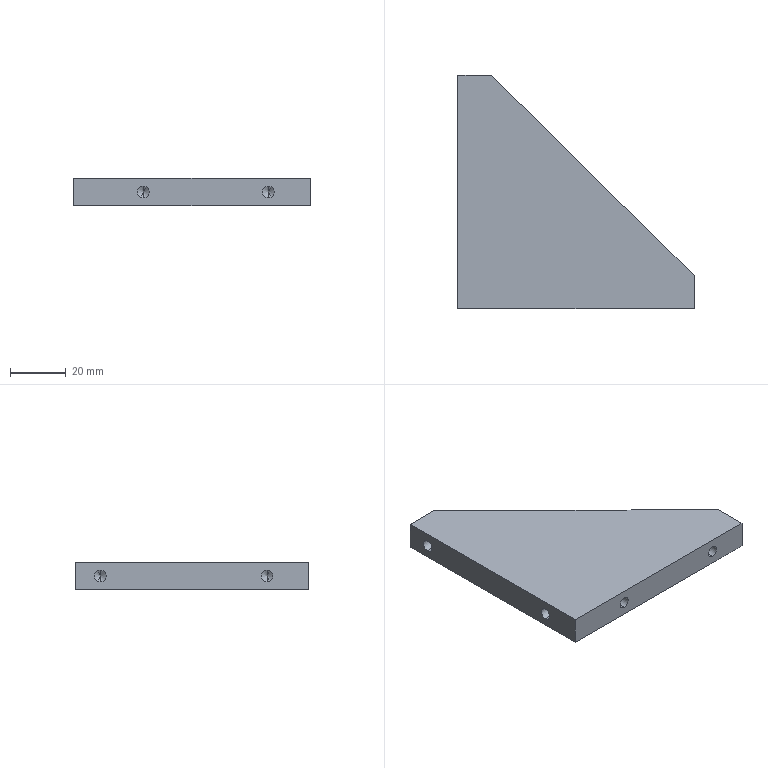Part | STEP file | 2047 Reinforcing rib 3 | 1 solid | 23 faces | box 85 x 84 x 10 mm | volume 44321 mm3 | cylinder 8 | cone 8 | plane 7 | commonest cylinder face diameters 4.2 x8